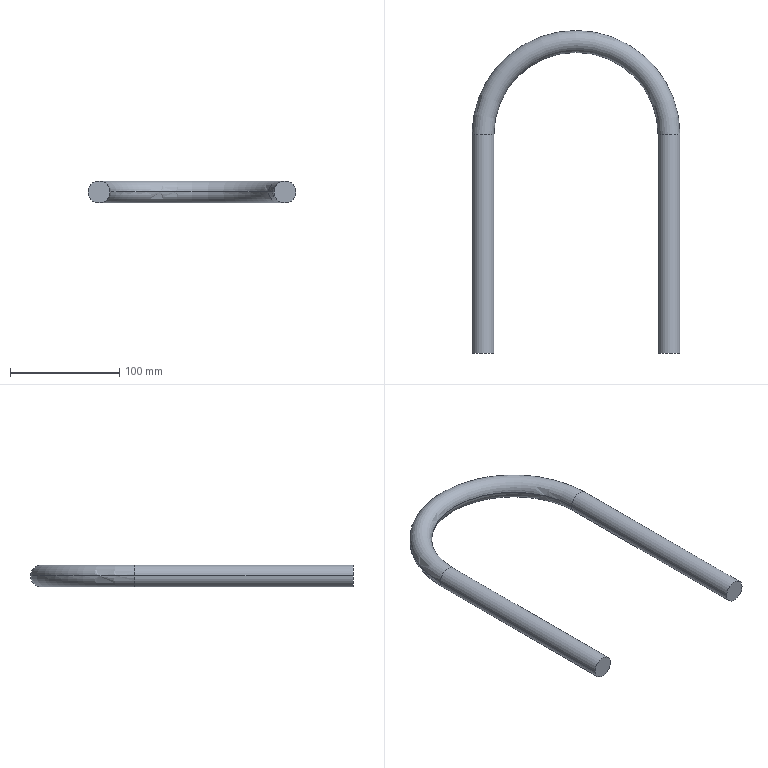Part | STEP file | Hanger_Default<As machined> | 3 solids | 12 faces | box 190 x 295 x 20 mm | volume 209555 mm3 | plane 6 | cylinder 4 | torus 2 | commonest cylinder face diameters 20 x4
STEP:
#1=CARTESIAN_POINT('',(0.,0.,0.));
#2=DIRECTION('',(0.,0.,1.));
#3=DIRECTION('',(1.,0.,0.));
#4=AXIS2_PLACEMENT_3D('',#1,#2,#3);
#5=CARTESIAN_POINT('',(-95.,200.,0.));
#6=VERTEX_POINT('',#5);
#7=CARTESIAN_POINT('',(-75.,200.,0.));
#8=VERTEX_POINT('',#7);
#9=CARTESIAN_POINT('',(-85.,200.,0.));
#10=DIRECTION('',(0.,1.,0.));
#11=DIRECTION('',(-1.,0.,0.));
#12=AXIS2_PLACEMENT_3D('',#9,#10,#11);
#13=CIRCLE('',#12,10.);
#14=CARTESIAN_POINT('',(-85.,200.,0.));
#15=DIRECTION('',(0.,-1.,0.));
#16=DIRECTION('',(1.,0.,0.));
#17=AXIS2_PLACEMENT_3D('',#14,#15,#16);
#18=CYLINDRICAL_SURFACE('',#17,10.);
#19=CARTESIAN_POINT('',(3.142,0.));
#20=DIRECTION('',(-1.,0.));
#21=VECTOR('',#20,1.);
#22=LINE('',#19,#21);
#23=(GEOMETRIC_REPRESENTATION_CONTEXT(2)PARAMETRIC_REPRESENTATION_CONTEXT()REPRESENTATION_CONTEXT('',''));
#24=DEFINITIONAL_REPRESENTATION('',(#22),#23);
#25=PCURVE('',#18,#24);
#26=CARTESIAN_POINT('',(-85.,200.,0.));
#27=DIRECTION('',(0.,1.,0.));
#28=DIRECTION('',(-1.,0.,0.));
#29=AXIS2_PLACEMENT_3D('',#26,#27,#28);
#30=PLANE('',#29);
#31=CARTESIAN_POINT('',(0.,0.));
#32=DIRECTION('',(1.,0.));
#33=AXIS2_PLACEMENT_2D('',#31,#32);
#34=CIRCLE('',#33,10.);
#35=(GEOMETRIC_REPRESENTATION_CONTEXT(2)PARAMETRIC_REPRESENTATION_CONTEXT()REPRESENTATION_CONTEXT('',''));
#36=DEFINITIONAL_REPRESENTATION('',(#34),#35);
#37=PCURVE('',#30,#36);
#38=SURFACE_CURVE('',#13,(#25,#37),.PCURVE_S1.);
#39=EDGE_CURVE('',#6,#8,#38,.T.);
#40=ORIENTED_EDGE('',*,*,#39,.F.);
#41=CARTESIAN_POINT('',(-95.,0.,0.));
#42=VERTEX_POINT('',#41);
#43=CARTESIAN_POINT('',(-95.,200.,0.));
#44=DIRECTION('',(0.,-1.,0.));
#45=VECTOR('',#44,1.);
#46=LINE('',#43,#45);
#47=CARTESIAN_POINT('',(3.142,0.));
#48=DIRECTION('',(0.,1.));
#49=VECTOR('',#48,1.);
#50=LINE('',#47,#49);
#51=(GEOMETRIC_REPRESENTATION_CONTEXT(2)PARAMETRIC_REPRESENTATION_CONTEXT()REPRESENTATION_CONTEXT('',''));
#52=DEFINITIONAL_REPRESENTATION('',(#50),#51);
#53=PCURVE('',#18,#52);
#54=CARTESIAN_POINT('',(-85.,200.,0.));
#55=DIRECTION('',(0.,-1.,0.));
#56=DIRECTION('',(1.,0.,0.));
#57=AXIS2_PLACEMENT_3D('',#54,#55,#56);
#58=CYLINDRICAL_SURFACE('',#57,10.);
#59=CARTESIAN_POINT('',(3.142,0.));
#60=DIRECTION('',(0.,1.));
#61=VECTOR('',#60,1.);
#62=LINE('',#59,#61);
#63=(GEOMETRIC_REPRESENTATION_CONTEXT(2)PARAMETRIC_REPRESENTATION_CONTEXT()REPRESENTATION_CONTEXT('',''));
#64=DEFINITIONAL_REPRESENTATION('',(#62),#63);
#65=PCURVE('',#58,#64);
#66=SURFACE_CURVE('',#46,(#53,#65),.PCURVE_S1.);
#67=EDGE_CURVE('',#6,#42,#66,.T.);
#68=ORIENTED_EDGE('',*,*,#67,.T.);
#69=CARTESIAN_POINT('',(-75.,0.,0.));
#70=VERTEX_POINT('',#69);
#71=CARTESIAN_POINT('',(-85.,0.,0.));
#72=DIRECTION('',(0.,1.,0.));
#73=DIRECTION('',(-1.,0.,0.));
#74=AXIS2_PLACEMENT_3D('',#71,#72,#73);
#75=CIRCLE('',#74,10.);
#76=CARTESIAN_POINT('',(3.142,200.));
#77=DIRECTION('',(-1.,0.));
#78=VECTOR('',#77,1.);
#79=LINE('',#76,#78);
#80=(GEOMETRIC_REPRESENTATION_CONTEXT(2)PARAMETRIC_REPRESENTATION_CONTEXT()REPRESENTATION_CONTEXT('',''));
#81=DEFINITIONAL_REPRESENTATION('',(#79),#80);
#82=PCURVE('',#18,#81);
#83=CARTESIAN_POINT('',(-85.,0.,0.));
#84=DIRECTION('',(0.,1.,0.));
#85=DIRECTION('',(-1.,0.,0.));
#86=AXIS2_PLACEMENT_3D('',#83,#84,#85);
#87=PLANE('',#86);
#88=CARTESIAN_POINT('',(0.,0.));
#89=DIRECTION('',(1.,0.));
#90=AXIS2_PLACEMENT_2D('',#88,#89);
#91=CIRCLE('',#90,10.);
#92=(GEOMETRIC_REPRESENTATION_CONTEXT(2)PARAMETRIC_REPRESENTATION_CONTEXT()REPRESENTATION_CONTEXT('',''));
#93=DEFINITIONAL_REPRESENTATION('',(#91),#92);
#94=PCURVE('',#87,#93);
#95=SURFACE_CURVE('',#75,(#82,#94),.PCURVE_S1.);
#96=EDGE_CURVE('',#42,#70,#95,.T.);
#97=ORIENTED_EDGE('',*,*,#96,.T.);
#98=CARTESIAN_POINT('',(-75.,200.,0.));
#99=DIRECTION('',(0.,-1.,0.));
#100=VECTOR('',#99,1.);
#101=LINE('',#98,#100);
#102=CARTESIAN_POINT('',(0.,0.));
#103=DIRECTION('',(0.,1.));
#104=VECTOR('',#103,1.);
#105=LINE('',#102,#104);
#106=(GEOMETRIC_REPRESENTATION_CONTEXT(2)PARAMETRIC_REPRESENTATION_CONTEXT()REPRESENTATION_CONTEXT('',''));
#107=DEFINITIONAL_REPRESENTATION('',(#105),#106);
#108=PCURVE('',#18,#107);
#109=CARTESIAN_POINT('',(6.283,0.));
#110=DIRECTION('',(0.,1.));
#111=VECTOR('',#110,1.);
#112=LINE('',#109,#111);
#113=(GEOMETRIC_REPRESENTATION_CONTEXT(2)PARAMETRIC_REPRESENTATION_CONTEXT()REPRESENTATION_CONTEXT('',''));
#114=DEFINITIONAL_REPRESENTATION('',(#112),#113);
#115=PCURVE('',#58,#114);
#116=SURFACE_CURVE('',#101,(#108,#115),.PCURVE_S1.);
#117=EDGE_CURVE('',#8,#70,#116,.T.);
#118=ORIENTED_EDGE('',*,*,#117,.F.);
#119=EDGE_LOOP('',(#40,#68,#97,#118));
#120=FACE_BOUND('',#119,.T.);
#121=ADVANCED_FACE('',(#120),#18,.T.);
#122=ORIENTED_EDGE('',*,*,#67,.F.);
#123=CARTESIAN_POINT('',(-85.,200.,0.));
#124=DIRECTION('',(0.,1.,0.));
#125=DIRECTION('',(-1.,0.,0.));
#126=AXIS2_PLACEMENT_3D('',#123,#124,#125);
#127=CIRCLE('',#126,10.);
#128=CARTESIAN_POINT('',(9.425,0.));
#129=DIRECTION('',(-1.,0.));
#130=VECTOR('',#129,1.);
#131=LINE('',#128,#130);
#132=(GEOMETRIC_REPRESENTATION_CONTEXT(2)PARAMETRIC_REPRESENTATION_CONTEXT()REPRESENTATION_CONTEXT('',''));
#133=DEFINITIONAL_REPRESENTATION('',(#131),#132);
#134=PCURVE('',#58,#133);
#135=CARTESIAN_POINT('',(0.,0.));
#136=DIRECTION('',(1.,0.));
#137=AXIS2_PLACEMENT_2D('',#135,#136);
#138=CIRCLE('',#137,10.);
#139=(GEOMETRIC_REPRESENTATION_CONTEXT(2)PARAMETRIC_REPRESENTATION_CONTEXT()REPRESENTATION_CONTEXT('',''));
#140=DEFINITIONAL_REPRESENTATION('',(#138),#139);
#141=PCURVE('',#30,#140);
#142=SURFACE_CURVE('',#127,(#134,#141),.PCURVE_S1.);
#143=EDGE_CURVE('',#8,#6,#142,.T.);
#144=ORIENTED_EDGE('',*,*,#143,.F.);
#145=ORIENTED_EDGE('',*,*,#117,.T.);
#146=CARTESIAN_POINT('',(-85.,0.,0.));
#147=DIRECTION('',(0.,1.,0.));
#148=DIRECTION('',(-1.,0.,0.));
#149=AXIS2_PLACEMENT_3D('',#146,#147,#148);
#150=CIRCLE('',#149,10.);
#151=CARTESIAN_POINT('',(9.425,200.));
#152=DIRECTION('',(-1.,0.));
#153=VECTOR('',#152,1.);
#154=LINE('',#151,#153);
#155=(GEOMETRIC_REPRESENTATION_CONTEXT(2)PARAMETRIC_REPRESENTATION_CONTEXT()REPRESENTATION_CONTEXT('',''));
#156=DEFINITIONAL_REPRESENTATION('',(#154),#155);
#157=PCURVE('',#58,#156);
#158=CARTESIAN_POINT('',(0.,0.));
#159=DIRECTION('',(1.,0.));
#160=AXIS2_PLACEMENT_2D('',#158,#159);
#161=CIRCLE('',#160,10.);
#162=(GEOMETRIC_REPRESENTATION_CONTEXT(2)PARAMETRIC_REPRESENTATION_CONTEXT()REPRESENTATION_CONTEXT('',''));
#163=DEFINITIONAL_REPRESENTATION('',(#161),#162);
#164=PCURVE('',#87,#163);
#165=SURFACE_CURVE('',#150,(#157,#164),.PCURVE_S1.);
#166=EDGE_CURVE('',#70,#42,#165,.T.);
#167=ORIENTED_EDGE('',*,*,#166,.T.);
#168=EDGE_LOOP('',(#122,#144,#145,#167));
#169=FACE_BOUND('',#168,.T.);
#170=ADVANCED_FACE('',(#169),#58,.T.);
#171=ORIENTED_EDGE('',*,*,#166,.F.);
#172=ORIENTED_EDGE('',*,*,#96,.F.);
#173=EDGE_LOOP('',(#171,#172));
#174=FACE_BOUND('',#173,.T.);
#175=ADVANCED_FACE('',(#174),#87,.F.);
#176=ORIENTED_EDGE('',*,*,#143,.T.);
#177=ORIENTED_EDGE('',*,*,#39,.T.);
#178=EDGE_LOOP('',(#176,#177));
#179=FACE_BOUND('',#178,.T.);
#180=ADVANCED_FACE('',(#179),#30,.T.);
#181=CLOSED_SHELL('',(#121,#170,#175,#180));
#182=MANIFOLD_SOLID_BREP('',#181);
#183=CARTESIAN_POINT('',(95.,200.,0.));
#184=VERTEX_POINT('',#183);
#185=CARTESIAN_POINT('',(75.,200.,0.));
#186=VERTEX_POINT('',#185);
#187=CARTESIAN_POINT('',(85.,200.,0.));
#188=DIRECTION('',(0.,-1.,0.));
#189=DIRECTION('',(1.,0.,0.));
#190=AXIS2_PLACEMENT_3D('',#187,#188,#189);
#191=CIRCLE('',#190,10.);
#192=CARTESIAN_POINT('',(0.,200.,0.));
#193=DIRECTION('',(0.,0.,1.));
#194=DIRECTION('',(1.,0.,0.));
#195=AXIS2_PLACEMENT_3D('',#192,#193,#194);
#196=TOROIDAL_SURFACE('',#195,85.,10.);
#197=CARTESIAN_POINT('',(0.,0.));
#198=DIRECTION('',(0.,1.));
#199=VECTOR('',#198,1.);
#200=LINE('',#197,#199);
#201=(GEOMETRIC_REPRESENTATION_CONTEXT(2)PARAMETRIC_REPRESENTATION_CONTEXT()REPRESENTATION_CONTEXT('',''));
#202=DEFINITIONAL_REPRESENTATION('',(#200),#201);
#203=PCURVE('',#196,#202);
#204=CARTESIAN_POINT('',(85.,200.,0.));
#205=DIRECTION('',(0.,-1.,0.));
#206=DIRECTION('',(1.,0.,0.));
#207=AXIS2_PLACEMENT_3D('',#204,#205,#206);
#208=PLANE('',#207);
#209=CARTESIAN_POINT('',(0.,0.));
#210=DIRECTION('',(1.,0.));
#211=AXIS2_PLACEMENT_2D('',#209,#210);
#212=CIRCLE('',#211,10.);
#213=(GEOMETRIC_REPRESENTATION_CONTEXT(2)PARAMETRIC_REPRESENTATION_CONTEXT()REPRESENTATION_CONTEXT('',''));
#214=DEFINITIONAL_REPRESENTATION('',(#212),#213);
#215=PCURVE('',#208,#214);
#216=SURFACE_CURVE('',#191,(#203,#215),.PCURVE_S1.);
#217=EDGE_CURVE('',#184,#186,#216,.T.);
#218=ORIENTED_EDGE('',*,*,#217,.F.);
#219=CARTESIAN_POINT('',(-95.,200.,0.));
#220=VERTEX_POINT('',#219);
#221=CARTESIAN_POINT('',(0.,200.,0.));
#222=DIRECTION('',(0.,0.,1.));
#223=DIRECTION('',(1.,0.,0.));
#224=AXIS2_PLACEMENT_3D('',#221,#222,#223);
#225=CIRCLE('',#224,95.);
#226=CARTESIAN_POINT('',(0.,0.));
#227=DIRECTION('',(1.,0.));
#228=VECTOR('',#227,1.);
#229=LINE('',#226,#228);
#230=(GEOMETRIC_REPRESENTATION_CONTEXT(2)PARAMETRIC_REPRESENTATION_CONTEXT()REPRESENTATION_CONTEXT('',''));
#231=DEFINITIONAL_REPRESENTATION('',(#229),#230);
#232=PCURVE('',#196,#231);
#233=CARTESIAN_POINT('',(0.,200.,0.));
#234=DIRECTION('',(0.,0.,1.));
#235=DIRECTION('',(1.,0.,0.));
#236=AXIS2_PLACEMENT_3D('',#233,#234,#235);
#237=TOROIDAL_SURFACE('',#236,85.,10.);
#238=CARTESIAN_POINT('',(0.,6.283));
#239=DIRECTION('',(1.,0.));
#240=VECTOR('',#239,1.);
#241=LINE('',#238,#240);
#242=(GEOMETRIC_REPRESENTATION_CONTEXT(2)PARAMETRIC_REPRESENTATION_CONTEXT()REPRESENTATION_CONTEXT('',''));
#243=DEFINITIONAL_REPRESENTATION('',(#241),#242);
#244=PCURVE('',#237,#243);
#245=SURFACE_CURVE('',#225,(#232,#244),.PCURVE_S1.);
#246=EDGE_CURVE('',#184,#220,#245,.T.);
#247=ORIENTED_EDGE('',*,*,#246,.T.);
#248=CARTESIAN_POINT('',(-75.,200.,0.));
#249=VERTEX_POINT('',#248);
#250=CARTESIAN_POINT('',(-85.,200.,0.));
#251=DIRECTION('',(0.,-1.,0.));
#252=DIRECTION('',(1.,0.,0.));
#253=AXIS2_PLACEMENT_3D('',#250,#251,#252);
#254=CIRCLE('',#253,10.);
#255=CARTESIAN_POINT('',(3.142,3.142));
#256=DIRECTION('',(0.,-1.));
#257=VECTOR('',#256,1.);
#258=LINE('',#255,#257);
#259=(GEOMETRIC_REPRESENTATION_CONTEXT(2)PARAMETRIC_REPRESENTATION_CONTEXT()REPRESENTATION_CONTEXT('',''));
#260=DEFINITIONAL_REPRESENTATION('',(#258),#259);
#261=PCURVE('',#196,#260);
#262=CARTESIAN_POINT('',(-85.,200.,0.));
#263=DIRECTION('',(0.,-1.,0.));
#264=DIRECTION('',(1.,0.,0.));
#265=AXIS2_PLACEMENT_3D('',#262,#263,#264);
#266=PLANE('',#265);
#267=CARTESIAN_POINT('',(0.,0.));
#268=DIRECTION('',(1.,0.));
#269=AXIS2_PLACEMENT_2D('',#267,#268);
#270=CIRCLE('',#269,10.);
#271=(GEOMETRIC_REPRESENTATION_CONTEXT(2)PARAMETRIC_REPRESENTATION_CONTEXT()REPRESENTATION_CONTEXT('',''));
#272=DEFINITIONAL_REPRESENTATION('',(#270),#271);
#273=PCURVE('',#266,#272);
#274=SURFACE_CURVE('',#254,(#261,#273),.PCURVE_S1.);
#275=EDGE_CURVE('',#249,#220,#274,.T.);
#276=ORIENTED_EDGE('',*,*,#275,.F.);
#277=CARTESIAN_POINT('',(0.,200.,0.));
#278=DIRECTION('',(0.,0.,1.));
#279=DIRECTION('',(1.,0.,0.));
#280=AXIS2_PLACEMENT_3D('',#277,#278,#279);
#281=CIRCLE('',#280,75.);
#282=CARTESIAN_POINT('',(0.,3.142));
#283=DIRECTION('',(1.,0.));
#284=VECTOR('',#283,1.);
#285=LINE('',#282,#284);
#286=(GEOMETRIC_REPRESENTATION_CONTEXT(2)PARAMETRIC_REPRESENTATION_CONTEXT()REPRESENTATION_CONTEXT('',''));
#287=DEFINITIONAL_REPRESENTATION('',(#285),#286);
#288=PCURVE('',#196,#287);
#289=CARTESIAN_POINT('',(0.,3.142));
#290=DIRECTION('',(1.,0.));
#291=VECTOR('',#290,1.);
#292=LINE('',#289,#291);
#293=(GEOMETRIC_REPRESENTATION_CONTEXT(2)PARAMETRIC_REPRESENTATION_CONTEXT()REPRESENTATION_CONTEXT('',''));
#294=DEFINITIONAL_REPRESENTATION('',(#292),#293);
#295=PCURVE('',#237,#294);
#296=SURFACE_CURVE('',#281,(#288,#295),.PCURVE_S1.);
#297=EDGE_CURVE('',#186,#249,#296,.T.);
#298=ORIENTED_EDGE('',*,*,#297,.F.);
#299=EDGE_LOOP('',(#218,#247,#276,#298));
#300=FACE_BOUND('',#299,.T.);
#301=ADVANCED_FACE('',(#300),#196,.T.);
#302=ORIENTED_EDGE('',*,*,#246,.F.);
#303=CARTESIAN_POINT('',(85.,200.,0.));
#304=DIRECTION('',(0.,-1.,0.));
#305=DIRECTION('',(1.,0.,0.));
#306=AXIS2_PLACEMENT_3D('',#303,#304,#305);
#307=CIRCLE('',#306,10.);
#308=CARTESIAN_POINT('',(0.,0.));
#309=DIRECTION('',(0.,1.));
#310=VECTOR('',#309,1.);
#311=LINE('',#308,#310);
#312=(GEOMETRIC_REPRESENTATION_CONTEXT(2)PARAMETRIC_REPRESENTATION_CONTEXT()REPRESENTATION_CONTEXT('',''));
#313=DEFINITIONAL_REPRESENTATION('',(#311),#312);
#314=PCURVE('',#237,#313);
#315=CARTESIAN_POINT('',(0.,0.));
#316=DIRECTION('',(1.,0.));
#317=AXIS2_PLACEMENT_2D('',#315,#316);
#318=CIRCLE('',#317,10.);
#319=(GEOMETRIC_REPRESENTATION_CONTEXT(2)PARAMETRIC_REPRESENTATION_CONTEXT()REPRESENTATION_CONTEXT('',''));
#320=DEFINITIONAL_REPRESENTATION('',(#318),#319);
#321=PCURVE('',#208,#320);
#322=SURFACE_CURVE('',#307,(#314,#321),.PCURVE_S1.);
#323=EDGE_CURVE('',#186,#184,#322,.T.);
#324=ORIENTED_EDGE('',*,*,#323,.F.);
#325=ORIENTED_EDGE('',*,*,#297,.T.);
#326=CARTESIAN_POINT('',(-85.,200.,0.));
#327=DIRECTION('',(0.,-1.,0.));
#328=DIRECTION('',(1.,0.,0.));
#329=AXIS2_PLACEMENT_3D('',#326,#327,#328);
#330=CIRCLE('',#329,10.);
#331=CARTESIAN_POINT('',(3.142,9.425));
#332=DIRECTION('',(0.,-1.));
#333=VECTOR('',#332,1.);
#334=LINE('',#331,#333);
#335=(GEOMETRIC_REPRESENTATION_CONTEXT(2)PARAMETRIC_REPRESENTATION_CONTEXT()REPRESENTATION_CONTEXT('',''));
#336=DEFINITIONAL_REPRESENTATION('',(#334),#335);
#337=PCURVE('',#237,#336);
#338=CARTESIAN_POINT('',(0.,0.));
#339=DIRECTION('',(1.,0.));
#340=AXIS2_PLACEMENT_2D('',#338,#339);
#341=CIRCLE('',#340,10.);
#342=(GEOMETRIC_REPRESENTATION_CONTEXT(2)PARAMETRIC_REPRESENTATION_CONTEXT()REPRESENTATION_CONTEXT('',''));
#343=DEFINITIONAL_REPRESENTATION('',(#341),#342);
#344=PCURVE('',#266,#343);
#345=SURFACE_CURVE('',#330,(#337,#344),.PCURVE_S1.);
#346=EDGE_CURVE('',#220,#249,#345,.T.);
#347=ORIENTED_EDGE('',*,*,#346,.F.);
#348=EDGE_LOOP('',(#302,#324,#325,#347));
#349=FACE_BOUND('',#348,.T.);
#350=ADVANCED_FACE('',(#349),#237,.T.);
#351=ORIENTED_EDGE('',*,*,#323,.T.);
#352=ORIENTED_EDGE('',*,*,#217,.T.);
#353=EDGE_LOOP('',(#351,#352));
#354=FACE_BOUND('',#353,.T.);
#355=ADVANCED_FACE('',(#354),#208,.T.);
#356=ORIENTED_EDGE('',*,*,#275,.T.);
#357=ORIENTED_EDGE('',*,*,#346,.T.);
#358=EDGE_LOOP('',(#356,#357));
#359=FACE_BOUND('',#358,.T.);
#360=ADVANCED_FACE('',(#359),#266,.T.);
#361=CLOSED_SHELL('',(#301,#350,#355,#360));
#362=MANIFOLD_SOLID_BREP('',#361);
#363=CARTESIAN_POINT('',(95.,0.,0.));
#364=VERTEX_POINT('',#363);
#365=CARTESIAN_POINT('',(75.,0.,0.));
#366=VERTEX_POINT('',#365);
#367=CARTESIAN_POINT('',(85.,0.,0.));
#368=DIRECTION('',(0.,-1.,0.));
#369=DIRECTION('',(1.,0.,0.));
#370=AXIS2_PLACEMENT_3D('',#367,#368,#369);
#371=CIRCLE('',#370,10.);
#372=CARTESIAN_POINT('',(85.,0.,0.));
#373=DIRECTION('',(0.,1.,0.));
#374=DIRECTION('',(-1.,0.,0.));
#375=AXIS2_PLACEMENT_3D('',#372,#373,#374);
#376=CYLINDRICAL_SURFACE('',#375,10.);
#377=CARTESIAN_POINT('',(3.142,0.));
#378=DIRECTION('',(-1.,0.));
#379=VECTOR('',#378,1.);
#380=LINE('',#377,#379);
#381=(GEOMETRIC_REPRESENTATION_CONTEXT(2)PARAMETRIC_REPRESENTATION_CONTEXT()REPRESENTATION_CONTEXT('',''));
#382=DEFINITIONAL_REPRESENTATION('',(#380),#381);
#383=PCURVE('',#376,#382);
#384=CARTESIAN_POINT('',(85.,0.,0.));
#385=DIRECTION('',(0.,-1.,0.));
#386=DIRECTION('',(1.,0.,0.));
#387=AXIS2_PLACEMENT_3D('',#384,#385,#386);
#388=PLANE('',#387);
#389=CARTESIAN_POINT('',(0.,0.));
#390=DIRECTION('',(1.,0.));
#391=AXIS2_PLACEMENT_2D('',#389,#390);
#392=CIRCLE('',#391,10.);
#393=(GEOMETRIC_REPRESENTATION_CONTEXT(2)PARAMETRIC_REPRESENTATION_CONTEXT()REPRESENTATION_CONTEXT('',''));
#394=DEFINITIONAL_REPRESENTATION('',(#392),#393);
#395=PCURVE('',#388,#394);
#396=SURFACE_CURVE('',#371,(#383,#395),.PCURVE_S1.);
#397=EDGE_CURVE('',#364,#366,#396,.T.);
#398=ORIENTED_EDGE('',*,*,#397,.F.);
#399=CARTESIAN_POINT('',(95.,200.,0.));
#400=VERTEX_POINT('',#399);
#401=CARTESIAN_POINT('',(95.,0.,0.));
#402=DIRECTION('',(0.,1.,0.));
#403=VECTOR('',#402,1.);
#404=LINE('',#401,#403);
#405=CARTESIAN_POINT('',(3.142,0.));
#406=DIRECTION('',(0.,1.));
#407=VECTOR('',#406,1.);
#408=LINE('',#405,#407);
#409=(GEOMETRIC_REPRESENTATION_CONTEXT(2)PARAMETRIC_REPRESENTATION_CONTEXT()REPRESENTATION_CONTEXT('',''));
#410=DEFINITIONAL_REPRESENTATION('',(#408),#409);
#411=PCURVE('',#376,#410);
#412=CARTESIAN_POINT('',(85.,0.,0.));
#413=DIRECTION('',(0.,1.,0.));
#414=DIRECTION('',(-1.,0.,0.));
#415=AXIS2_PLACEMENT_3D('',#412,#413,#414);
#416=CYLINDRICAL_SURFACE('',#415,10.);
#417=CARTESIAN_POINT('',(3.142,0.));
#418=DIRECTION('',(0.,1.));
#419=VECTOR('',#418,1.);
#420=LINE('',#417,#419);
#421=(GEOMETRIC_REPRESENTATION_CONTEXT(2)PARAMETRIC_REPRESENTATION_CONTEXT()REPRESENTATION_CONTEXT('',''));
#422=DEFINITIONAL_REPRESENTATION('',(#420),#421);
#423=PCURVE('',#416,#422);
#424=SURFACE_CURVE('',#404,(#411,#423),.PCURVE_S1.);
#425=EDGE_CURVE('',#364,#400,#424,.T.);
#426=ORIENTED_EDGE('',*,*,#425,.T.);
#427=CARTESIAN_POINT('',(75.,200.,0.));
#428=VERTEX_POINT('',#427);
#429=CARTESIAN_POINT('',(85.,200.,0.));
#430=DIRECTION('',(0.,1.,0.));
#431=DIRECTION('',(-1.,0.,0.));
#432=AXIS2_PLACEMENT_3D('',#429,#430,#431);
#433=CIRCLE('',#432,10.);
#434=CARTESIAN_POINT('',(0.,200.));
#435=DIRECTION('',(1.,0.));
#436=VECTOR('',#435,1.);
#437=LINE('',#434,#436);
#438=(GEOMETRIC_REPRESENTATION_CONTEXT(2)PARAMETRIC_REPRESENTATION_CONTEXT()REPRESENTATION_CONTEXT('',''));
#439=DEFINITIONAL_REPRESENTATION('',(#437),#438);
#440=PCURVE('',#376,#439);
#441=CARTESIAN_POINT('',(85.,200.,0.));
#442=DIRECTION('',(0.,1.,0.));
#443=DIRECTION('',(-1.,0.,0.));
#444=AXIS2_PLACEMENT_3D('',#441,#442,#443);
#445=PLANE('',#444);
#446=CARTESIAN_POINT('',(0.,0.));
#447=DIRECTION('',(1.,0.));
#448=AXIS2_PLACEMENT_2D('',#446,#447);
#449=CIRCLE('',#448,10.);
#450=(GEOMETRIC_REPRESENTATION_CONTEXT(2)PARAMETRIC_REPRESENTATION_CONTEXT()REPRESENTATION_CONTEXT('',''));
#451=DEFINITIONAL_REPRESENTATION('',(#449),#450);
#452=PCURVE('',#445,#451);
#453=SURFACE_CURVE('',#433,(#440,#452),.PCURVE_S1.);
#454=EDGE_CURVE('',#428,#400,#453,.T.);
#455=ORIENTED_EDGE('',*,*,#454,.F.);
#456=CARTESIAN_POINT('',(75.,0.,0.));
#457=DIRECTION('',(0.,1.,0.));
#458=VECTOR('',#457,1.);
#459=LINE('',#456,#458);
#460=CARTESIAN_POINT('',(0.,0.));
#461=DIRECTION('',(0.,1.));
#462=VECTOR('',#461,1.);
#463=LINE('',#460,#462);
#464=(GEOMETRIC_REPRESENTATION_CONTEXT(2)PARAMETRIC_REPRESENTATION_CONTEXT()REPRESENTATION_CONTEXT('',''));
#465=DEFINITIONAL_REPRESENTATION('',(#463),#464);
#466=PCURVE('',#376,#465);
#467=CARTESIAN_POINT('',(6.283,0.));
#468=DIRECTION('',(0.,1.));
#469=VECTOR('',#468,1.);
#470=LINE('',#467,#469);
#471=(GEOMETRIC_REPRESENTATION_CONTEXT(2)PARAMETRIC_REPRESENTATION_CONTEXT()REPRESENTATION_CONTEXT('',''));
#472=DEFINITIONAL_REPRESENTATION('',(#470),#471);
#473=PCURVE('',#416,#472);
#474=SURFACE_CURVE('',#459,(#466,#473),.PCURVE_S1.);
#475=EDGE_CURVE('',#366,#428,#474,.T.);
#476=ORIENTED_EDGE('',*,*,#475,.F.);
#477=EDGE_LOOP('',(#398,#426,#455,#476));
#478=FACE_BOUND('',#477,.T.);
#479=ADVANCED_FACE('',(#478),#376,.T.);
#480=ORIENTED_EDGE('',*,*,#425,.F.);
#481=CARTESIAN_POINT('',(85.,0.,0.));
#482=DIRECTION('',(0.,-1.,0.));
#483=DIRECTION('',(1.,0.,0.));
#484=AXIS2_PLACEMENT_3D('',#481,#482,#483);
#485=CIRCLE('',#484,10.);
#486=CARTESIAN_POINT('',(9.425,0.));
#487=DIRECTION('',(-1.,0.));
#488=VECTOR('',#487,1.);
#489=LINE('',#486,#488);
#490=(GEOMETRIC_REPRESENTATION_CONTEXT(2)PARAMETRIC_REPRESENTATION_CONTEXT()REPRESENTATION_CONTEXT('',''));
#491=DEFINITIONAL_REPRESENTATION('',(#489),#490);
#492=PCURVE('',#416,#491);
#493=CARTESIAN_POINT('',(0.,0.));
#494=DIRECTION('',(1.,0.));
#495=AXIS2_PLACEMENT_2D('',#493,#494);
#496=CIRCLE('',#495,10.);
#497=(GEOMETRIC_REPRESENTATION_CONTEXT(2)PARAMETRIC_REPRESENTATION_CONTEXT()REPRESENTATION_CONTEXT('',''));
#498=DEFINITIONAL_REPRESENTATION('',(#496),#497);
#499=PCURVE('',#388,#498);
#500=SURFACE_CURVE('',#485,(#492,#499),.PCURVE_S1.);
#501=EDGE_CURVE('',#366,#364,#500,.T.);
#502=ORIENTED_EDGE('',*,*,#501,.F.);
#503=ORIENTED_EDGE('',*,*,#475,.T.);
#504=CARTESIAN_POINT('',(85.,200.,0.));
#505=DIRECTION('',(0.,1.,0.));
#506=DIRECTION('',(-1.,0.,0.));
#507=AXIS2_PLACEMENT_3D('',#504,#505,#506);
#508=CIRCLE('',#507,10.);
#509=CARTESIAN_POINT('',(0.,200.));
#510=DIRECTION('',(1.,0.));
#511=VECTOR('',#510,1.);
#512=LINE('',#509,#511);
#513=(GEOMETRIC_REPRESENTATION_CONTEXT(2)PARAMETRIC_REPRESENTATION_CONTEXT()REPRESENTATION_CONTEXT('',''));
#514=DEFINITIONAL_REPRESENTATION('',(#512),#513);
#515=PCURVE('',#416,#514);
#516=CARTESIAN_POINT('',(0.,0.));
#517=DIRECTION('',(1.,0.));
#518=AXIS2_PLACEMENT_2D('',#516,#517);
#519=CIRCLE('',#518,10.);
#520=(GEOMETRIC_REPRESENTATION_CONTEXT(2)PARAMETRIC_REPRESENTATION_CONTEXT()REPRESENTATION_CONTEXT('',''));
#521=DEFINITIONAL_REPRESENTATION('',(#519),#520);
#522=PCURVE('',#445,#521);
#523=SURFACE_CURVE('',#508,(#515,#522),.PCURVE_S1.);
#524=EDGE_CURVE('',#400,#428,#523,.T.);
#525=ORIENTED_EDGE('',*,*,#524,.F.);
#526=EDGE_LOOP('',(#480,#502,#503,#525));
#527=FACE_BOUND('',#526,.T.);
#528=ADVANCED_FACE('',(#527),#416,.T.);
#529=ORIENTED_EDGE('',*,*,#501,.T.);
#530=ORIENTED_EDGE('',*,*,#397,.T.);
#531=EDGE_LOOP('',(#529,#530));
#532=FACE_BOUND('',#531,.T.);
#533=ADVANCED_FACE('',(#532),#388,.T.);
#534=ORIENTED_EDGE('',*,*,#454,.T.);
#535=ORIENTED_EDGE('',*,*,#524,.T.);
#536=EDGE_LOOP('',(#534,#535));
#537=FACE_BOUND('',#536,.T.);
#538=ADVANCED_FACE('',(#537),#445,.T.);
#539=CLOSED_SHELL('',(#479,#528,#533,#538));
#540=MANIFOLD_SOLID_BREP('',#539);
#541=(LENGTH_UNIT()NAMED_UNIT(*)SI_UNIT(.MILLI.,.METRE.));
#542=UNCERTAINTY_MEASURE_WITH_UNIT(LENGTH_MEASURE(0.0000001),#541,'','');
#543=(NAMED_UNIT(*)PLANE_ANGLE_UNIT()SI_UNIT($,.RADIAN.));
#544=(NAMED_UNIT(*)SI_UNIT($,.STERADIAN.)SOLID_ANGLE_UNIT());
#545=(GEOMETRIC_REPRESENTATION_CONTEXT(3)GLOBAL_UNCERTAINTY_ASSIGNED_CONTEXT((#542))GLOBAL_UNIT_ASSIGNED_CONTEXT((#541,#543,#544))REPRESENTATION_CONTEXT('',''));
#546=SHAPE_REPRESENTATION('',(#4,#182,#362,#540),#545);